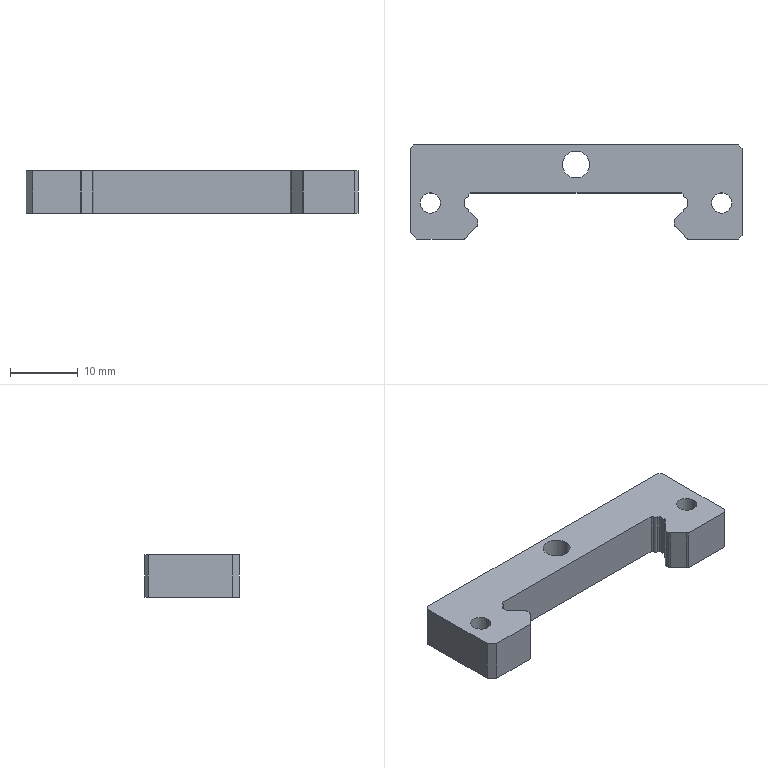Part | SolidWorks | features BaseBody 1 | 1 solid | 48 faces | box 49 x 13.9 x 6.3 mm | volume 2782 mm3 | plane 26 | cylinder 22 | commonest cylinder face diameters 1 x10 0.77 x6 3 x4 4 x2